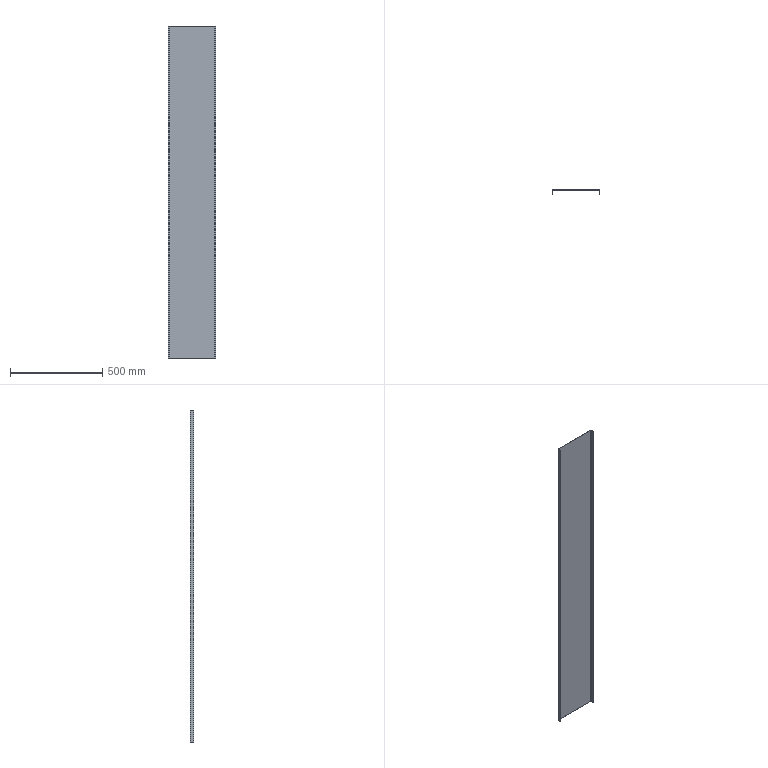Part | STEP file | 750038225 | 1 solid | 14 faces | box 255 x 21.5 x 1800 mm | volume 791285 mm3 | plane 10 | cylinder 4 | commonest cylinder face diameters 3 x2 6 x2
STEP:
#1=CARTESIAN_POINT('',(124.5,0.,900.));
#2=VERTEX_POINT('',#1);
#3=CARTESIAN_POINT('',(-124.5,0.,900.));
#4=VERTEX_POINT('',#3);
#5=CARTESIAN_POINT('',(126.,0.,900.));
#6=DIRECTION('',(-1.,0.,0.));
#7=VECTOR('',#6,1000.);
#8=LINE('',#5,#7);
#9=EDGE_CURVE('',#2,#4,#8,.T.);
#10=ORIENTED_EDGE('',*,*,#9,.T.);
#11=CARTESIAN_POINT('',(-124.5,0.,-900.));
#12=VERTEX_POINT('',#11);
#13=CARTESIAN_POINT('',(-124.5,0.,900.));
#14=DIRECTION('',(0.,0.,-1.));
#15=VECTOR('',#14,1000.);
#16=LINE('',#13,#15);
#17=EDGE_CURVE('',#4,#12,#16,.T.);
#18=ORIENTED_EDGE('',*,*,#17,.T.);
#19=CARTESIAN_POINT('',(124.5,0.,-900.));
#20=VERTEX_POINT('',#19);
#21=CARTESIAN_POINT('',(126.,0.,-900.));
#22=DIRECTION('',(1.,0.,0.));
#23=VECTOR('',#22,1000.);
#24=LINE('',#21,#23);
#25=EDGE_CURVE('',#12,#20,#24,.T.);
#26=ORIENTED_EDGE('',*,*,#25,.T.);
#27=CARTESIAN_POINT('',(124.5,0.,900.));
#28=DIRECTION('',(0.,0.,1.));
#29=VECTOR('',#28,1000.);
#30=LINE('',#27,#29);
#31=EDGE_CURVE('',#20,#2,#30,.T.);
#32=ORIENTED_EDGE('',*,*,#31,.T.);
#33=EDGE_LOOP('',(#10,#18,#26,#32));
#34=FACE_OUTER_BOUND('',#33,.T.);
#35=CARTESIAN_POINT('',(126.,0.,900.));
#36=DIRECTION('',(0.,-1.,0.));
#37=DIRECTION('',(1.,0.,0.));
#38=AXIS2_PLACEMENT_3D('',#35,#36,#37);
#39=PLANE('',#38);
#40=ADVANCED_FACE('',(#34),#39,.T.);
#41=ORIENTED_EDGE('',*,*,#17,.F.);
#42=CARTESIAN_POINT('',(-126.,-1.5,900.));
#43=VERTEX_POINT('',#42);
#44=CARTESIAN_POINT('',(-124.5,-1.5,900.));
#45=DIRECTION('',(0.,0.,-1.));
#46=DIRECTION('',(-1.,0.,0.));
#47=AXIS2_PLACEMENT_3D('',#44,#45,#46);
#48=CIRCLE('',#47,1.5);
#49=EDGE_CURVE('',#43,#4,#48,.T.);
#50=ORIENTED_EDGE('',*,*,#49,.F.);
#51=CARTESIAN_POINT('',(-126.,-1.5,-900.));
#52=VERTEX_POINT('',#51);
#53=CARTESIAN_POINT('',(-126.,-1.5,900.));
#54=DIRECTION('',(0.,0.,1.));
#55=VECTOR('',#54,1000.);
#56=LINE('',#53,#55);
#57=EDGE_CURVE('',#52,#43,#56,.T.);
#58=ORIENTED_EDGE('',*,*,#57,.F.);
#59=CARTESIAN_POINT('',(-124.5,-1.5,-900.));
#60=DIRECTION('',(0.,0.,1.));
#61=DIRECTION('',(-1.,0.,0.));
#62=AXIS2_PLACEMENT_3D('',#59,#60,#61);
#63=CIRCLE('',#62,1.5);
#64=EDGE_CURVE('',#12,#52,#63,.T.);
#65=ORIENTED_EDGE('',*,*,#64,.F.);
#66=EDGE_LOOP('',(#41,#50,#58,#65));
#67=FACE_OUTER_BOUND('',#66,.T.);
#68=CARTESIAN_POINT('',(-124.5,-1.5,900.));
#69=DIRECTION('',(0.,0.,-1.));
#70=DIRECTION('',(-1.,0.,0.));
#71=AXIS2_PLACEMENT_3D('',#68,#69,#70);
#72=CYLINDRICAL_SURFACE('',#71,1.5);
#73=ADVANCED_FACE('',(#67),#72,.F.);
#74=CARTESIAN_POINT('',(-127.5,-1.5,900.));
#75=VERTEX_POINT('',#74);
#76=CARTESIAN_POINT('',(-127.5,-20.,900.));
#77=VERTEX_POINT('',#76);
#78=CARTESIAN_POINT('',(-127.5,0.,900.));
#79=DIRECTION('',(0.,-1.,0.));
#80=VECTOR('',#79,1000.);
#81=LINE('',#78,#80);
#82=EDGE_CURVE('',#75,#77,#81,.T.);
#83=ORIENTED_EDGE('',*,*,#82,.T.);
#84=CARTESIAN_POINT('',(-126.,-20.,900.));
#85=VERTEX_POINT('',#84);
#86=CARTESIAN_POINT('',(-126.,-20.,900.));
#87=DIRECTION('',(-1.,0.,0.));
#88=VECTOR('',#87,1000.);
#89=LINE('',#86,#88);
#90=EDGE_CURVE('',#85,#77,#89,.T.);
#91=ORIENTED_EDGE('',*,*,#90,.F.);
#92=CARTESIAN_POINT('',(-126.,0.,900.));
#93=DIRECTION('',(0.,1.,0.));
#94=VECTOR('',#93,1000.);
#95=LINE('',#92,#94);
#96=EDGE_CURVE('',#85,#43,#95,.T.);
#97=ORIENTED_EDGE('',*,*,#96,.T.);
#98=ORIENTED_EDGE('',*,*,#49,.T.);
#99=ORIENTED_EDGE('',*,*,#9,.F.);
#100=CARTESIAN_POINT('',(126.,-1.5,900.));
#101=VERTEX_POINT('',#100);
#102=CARTESIAN_POINT('',(124.5,-1.5,900.));
#103=DIRECTION('',(0.,0.,-1.));
#104=DIRECTION('',(-1.,0.,0.));
#105=AXIS2_PLACEMENT_3D('',#102,#103,#104);
#106=CIRCLE('',#105,1.5);
#107=EDGE_CURVE('',#2,#101,#106,.T.);
#108=ORIENTED_EDGE('',*,*,#107,.T.);
#109=CARTESIAN_POINT('',(126.,-20.,900.));
#110=VERTEX_POINT('',#109);
#111=CARTESIAN_POINT('',(126.,0.,900.));
#112=DIRECTION('',(0.,-1.,0.));
#113=VECTOR('',#112,1000.);
#114=LINE('',#111,#113);
#115=EDGE_CURVE('',#101,#110,#114,.T.);
#116=ORIENTED_EDGE('',*,*,#115,.T.);
#117=CARTESIAN_POINT('',(127.5,-20.,900.));
#118=VERTEX_POINT('',#117);
#119=CARTESIAN_POINT('',(126.,-20.,900.));
#120=DIRECTION('',(1.,0.,0.));
#121=VECTOR('',#120,1000.);
#122=LINE('',#119,#121);
#123=EDGE_CURVE('',#110,#118,#122,.T.);
#124=ORIENTED_EDGE('',*,*,#123,.T.);
#125=CARTESIAN_POINT('',(127.5,-1.5,900.));
#126=VERTEX_POINT('',#125);
#127=CARTESIAN_POINT('',(127.5,0.,900.));
#128=DIRECTION('',(0.,1.,0.));
#129=VECTOR('',#128,1000.);
#130=LINE('',#127,#129);
#131=EDGE_CURVE('',#118,#126,#130,.T.);
#132=ORIENTED_EDGE('',*,*,#131,.T.);
#133=CARTESIAN_POINT('',(124.5,1.5,900.));
#134=VERTEX_POINT('',#133);
#135=CARTESIAN_POINT('',(124.5,-1.5,900.));
#136=DIRECTION('',(0.,0.,1.));
#137=DIRECTION('',(-1.,0.,0.));
#138=AXIS2_PLACEMENT_3D('',#135,#136,#137);
#139=CIRCLE('',#138,3.);
#140=EDGE_CURVE('',#126,#134,#139,.T.);
#141=ORIENTED_EDGE('',*,*,#140,.T.);
#142=CARTESIAN_POINT('',(-124.5,1.5,900.));
#143=VERTEX_POINT('',#142);
#144=CARTESIAN_POINT('',(-126.,1.5,900.));
#145=DIRECTION('',(-1.,0.,0.));
#146=VECTOR('',#145,1000.);
#147=LINE('',#144,#146);
#148=EDGE_CURVE('',#134,#143,#147,.T.);
#149=ORIENTED_EDGE('',*,*,#148,.T.);
#150=CARTESIAN_POINT('',(-124.5,-1.5,900.));
#151=DIRECTION('',(0.,0.,1.));
#152=DIRECTION('',(-1.,0.,0.));
#153=AXIS2_PLACEMENT_3D('',#150,#151,#152);
#154=CIRCLE('',#153,3.);
#155=EDGE_CURVE('',#143,#75,#154,.T.);
#156=ORIENTED_EDGE('',*,*,#155,.T.);
#157=EDGE_LOOP('',(#83,#91,#97,#98,#99,#108,#116,#124,#132,#141,#149,#156));
#158=FACE_OUTER_BOUND('',#157,.T.);
#159=CARTESIAN_POINT('',(-126.,0.,900.));
#160=DIRECTION('',(0.,0.,1.));
#161=DIRECTION('',(1.,0.,0.));
#162=AXIS2_PLACEMENT_3D('',#159,#160,#161);
#163=PLANE('',#162);
#164=ADVANCED_FACE('',(#158),#163,.T.);
#165=CARTESIAN_POINT('',(126.,-1.5,-900.));
#166=VERTEX_POINT('',#165);
#167=CARTESIAN_POINT('',(126.,-1.5,900.));
#168=DIRECTION('',(0.,0.,-1.));
#169=VECTOR('',#168,1000.);
#170=LINE('',#167,#169);
#171=EDGE_CURVE('',#101,#166,#170,.T.);
#172=ORIENTED_EDGE('',*,*,#171,.F.);
#173=ORIENTED_EDGE('',*,*,#107,.F.);
#174=ORIENTED_EDGE('',*,*,#31,.F.);
#175=CARTESIAN_POINT('',(124.5,-1.5,-900.));
#176=DIRECTION('',(0.,0.,1.));
#177=DIRECTION('',(-1.,0.,0.));
#178=AXIS2_PLACEMENT_3D('',#175,#176,#177);
#179=CIRCLE('',#178,1.5);
#180=EDGE_CURVE('',#166,#20,#179,.T.);
#181=ORIENTED_EDGE('',*,*,#180,.F.);
#182=EDGE_LOOP('',(#172,#173,#174,#181));
#183=FACE_OUTER_BOUND('',#182,.T.);
#184=CARTESIAN_POINT('',(124.5,-1.5,900.));
#185=DIRECTION('',(0.,0.,-1.));
#186=DIRECTION('',(-1.,0.,0.));
#187=AXIS2_PLACEMENT_3D('',#184,#185,#186);
#188=CYLINDRICAL_SURFACE('',#187,1.5);
#189=ADVANCED_FACE('',(#183),#188,.F.);
#190=ORIENTED_EDGE('',*,*,#180,.T.);
#191=ORIENTED_EDGE('',*,*,#25,.F.);
#192=ORIENTED_EDGE('',*,*,#64,.T.);
#193=CARTESIAN_POINT('',(-126.,-20.,-900.));
#194=VERTEX_POINT('',#193);
#195=CARTESIAN_POINT('',(-126.,-20.,-900.));
#196=DIRECTION('',(0.,1.,0.));
#197=VECTOR('',#196,1000.);
#198=LINE('',#195,#197);
#199=EDGE_CURVE('',#194,#52,#198,.T.);
#200=ORIENTED_EDGE('',*,*,#199,.F.);
#201=CARTESIAN_POINT('',(-127.5,-20.,-900.));
#202=VERTEX_POINT('',#201);
#203=CARTESIAN_POINT('',(-126.,-20.,-900.));
#204=DIRECTION('',(1.,0.,0.));
#205=VECTOR('',#204,1000.);
#206=LINE('',#203,#205);
#207=EDGE_CURVE('',#202,#194,#206,.T.);
#208=ORIENTED_EDGE('',*,*,#207,.F.);
#209=CARTESIAN_POINT('',(-127.5,-1.5,-900.));
#210=VERTEX_POINT('',#209);
#211=CARTESIAN_POINT('',(-127.5,-20.,-900.));
#212=DIRECTION('',(0.,-1.,0.));
#213=VECTOR('',#212,1000.);
#214=LINE('',#211,#213);
#215=EDGE_CURVE('',#210,#202,#214,.T.);
#216=ORIENTED_EDGE('',*,*,#215,.F.);
#217=CARTESIAN_POINT('',(-124.5,1.5,-900.));
#218=VERTEX_POINT('',#217);
#219=CARTESIAN_POINT('',(-124.5,-1.5,-900.));
#220=DIRECTION('',(0.,0.,1.));
#221=DIRECTION('',(-1.,0.,0.));
#222=AXIS2_PLACEMENT_3D('',#219,#220,#221);
#223=CIRCLE('',#222,3.);
#224=EDGE_CURVE('',#218,#210,#223,.T.);
#225=ORIENTED_EDGE('',*,*,#224,.F.);
#226=CARTESIAN_POINT('',(124.5,1.5,-900.));
#227=VERTEX_POINT('',#226);
#228=CARTESIAN_POINT('',(126.,1.5,-900.));
#229=DIRECTION('',(-1.,0.,0.));
#230=VECTOR('',#229,1000.);
#231=LINE('',#228,#230);
#232=EDGE_CURVE('',#227,#218,#231,.T.);
#233=ORIENTED_EDGE('',*,*,#232,.F.);
#234=CARTESIAN_POINT('',(127.5,-1.5,-900.));
#235=VERTEX_POINT('',#234);
#236=CARTESIAN_POINT('',(124.5,-1.5,-900.));
#237=DIRECTION('',(0.,0.,1.));
#238=DIRECTION('',(-1.,0.,0.));
#239=AXIS2_PLACEMENT_3D('',#236,#237,#238);
#240=CIRCLE('',#239,3.);
#241=EDGE_CURVE('',#235,#227,#240,.T.);
#242=ORIENTED_EDGE('',*,*,#241,.F.);
#243=CARTESIAN_POINT('',(127.5,-20.,-900.));
#244=VERTEX_POINT('',#243);
#245=CARTESIAN_POINT('',(127.5,-20.,-900.));
#246=DIRECTION('',(0.,1.,0.));
#247=VECTOR('',#246,1000.);
#248=LINE('',#245,#247);
#249=EDGE_CURVE('',#244,#235,#248,.T.);
#250=ORIENTED_EDGE('',*,*,#249,.F.);
#251=CARTESIAN_POINT('',(126.,-20.,-900.));
#252=VERTEX_POINT('',#251);
#253=CARTESIAN_POINT('',(126.,-20.,-900.));
#254=DIRECTION('',(-1.,0.,0.));
#255=VECTOR('',#254,1000.);
#256=LINE('',#253,#255);
#257=EDGE_CURVE('',#244,#252,#256,.T.);
#258=ORIENTED_EDGE('',*,*,#257,.T.);
#259=CARTESIAN_POINT('',(126.,-20.,-900.));
#260=DIRECTION('',(0.,-1.,0.));
#261=VECTOR('',#260,1000.);
#262=LINE('',#259,#261);
#263=EDGE_CURVE('',#166,#252,#262,.T.);
#264=ORIENTED_EDGE('',*,*,#263,.F.);
#265=EDGE_LOOP('',(#190,#191,#192,#200,#208,#216,#225,#233,#242,#250,#258,#264));
#266=FACE_OUTER_BOUND('',#265,.T.);
#267=CARTESIAN_POINT('',(126.,-20.,-900.));
#268=DIRECTION('',(0.,0.,1.));
#269=DIRECTION('',(1.,0.,0.));
#270=AXIS2_PLACEMENT_3D('',#267,#268,#269);
#271=PLANE('',#270);
#272=ADVANCED_FACE('',(#266),#271,.F.);
#273=ORIENTED_EDGE('',*,*,#96,.F.);
#274=CARTESIAN_POINT('',(-126.,-20.,900.));
#275=DIRECTION('',(0.,0.,-1.));
#276=VECTOR('',#275,1000.);
#277=LINE('',#274,#276);
#278=EDGE_CURVE('',#85,#194,#277,.T.);
#279=ORIENTED_EDGE('',*,*,#278,.T.);
#280=ORIENTED_EDGE('',*,*,#199,.T.);
#281=ORIENTED_EDGE('',*,*,#57,.T.);
#282=EDGE_LOOP('',(#273,#279,#280,#281));
#283=FACE_OUTER_BOUND('',#282,.T.);
#284=CARTESIAN_POINT('',(-126.,0.,900.));
#285=DIRECTION('',(1.,0.,0.));
#286=DIRECTION('',(0.,0.,-1.));
#287=AXIS2_PLACEMENT_3D('',#284,#285,#286);
#288=PLANE('',#287);
#289=ADVANCED_FACE('',(#283),#288,.T.);
#290=CARTESIAN_POINT('',(-127.5,-20.,900.));
#291=DIRECTION('',(0.,0.,-1.));
#292=VECTOR('',#291,1000.);
#293=LINE('',#290,#292);
#294=EDGE_CURVE('',#77,#202,#293,.T.);
#295=ORIENTED_EDGE('',*,*,#294,.F.);
#296=ORIENTED_EDGE('',*,*,#82,.F.);
#297=CARTESIAN_POINT('',(-127.5,-1.5,900.));
#298=DIRECTION('',(0.,0.,1.));
#299=VECTOR('',#298,1000.);
#300=LINE('',#297,#299);
#301=EDGE_CURVE('',#210,#75,#300,.T.);
#302=ORIENTED_EDGE('',*,*,#301,.F.);
#303=ORIENTED_EDGE('',*,*,#215,.T.);
#304=EDGE_LOOP('',(#295,#296,#302,#303));
#305=FACE_OUTER_BOUND('',#304,.T.);
#306=CARTESIAN_POINT('',(-127.5,0.,900.));
#307=DIRECTION('',(1.,0.,0.));
#308=DIRECTION('',(0.,0.,-1.));
#309=AXIS2_PLACEMENT_3D('',#306,#307,#308);
#310=PLANE('',#309);
#311=ADVANCED_FACE('',(#305),#310,.F.);
#312=ORIENTED_EDGE('',*,*,#155,.F.);
#313=CARTESIAN_POINT('',(-124.5,1.5,900.));
#314=DIRECTION('',(0.,0.,-1.));
#315=VECTOR('',#314,1000.);
#316=LINE('',#313,#315);
#317=EDGE_CURVE('',#143,#218,#316,.T.);
#318=ORIENTED_EDGE('',*,*,#317,.T.);
#319=ORIENTED_EDGE('',*,*,#224,.T.);
#320=ORIENTED_EDGE('',*,*,#301,.T.);
#321=EDGE_LOOP('',(#312,#318,#319,#320));
#322=FACE_OUTER_BOUND('',#321,.T.);
#323=CARTESIAN_POINT('',(-124.5,-1.5,900.));
#324=DIRECTION('',(0.,0.,-1.));
#325=DIRECTION('',(-1.,0.,0.));
#326=AXIS2_PLACEMENT_3D('',#323,#324,#325);
#327=CYLINDRICAL_SURFACE('',#326,3.);
#328=ADVANCED_FACE('',(#322),#327,.T.);
#329=ORIENTED_EDGE('',*,*,#317,.F.);
#330=ORIENTED_EDGE('',*,*,#148,.F.);
#331=CARTESIAN_POINT('',(124.5,1.5,900.));
#332=DIRECTION('',(0.,0.,1.));
#333=VECTOR('',#332,1000.);
#334=LINE('',#331,#333);
#335=EDGE_CURVE('',#227,#134,#334,.T.);
#336=ORIENTED_EDGE('',*,*,#335,.F.);
#337=ORIENTED_EDGE('',*,*,#232,.T.);
#338=EDGE_LOOP('',(#329,#330,#336,#337));
#339=FACE_OUTER_BOUND('',#338,.T.);
#340=CARTESIAN_POINT('',(126.,1.5,900.));
#341=DIRECTION('',(0.,-1.,0.));
#342=DIRECTION('',(1.,0.,0.));
#343=AXIS2_PLACEMENT_3D('',#340,#341,#342);
#344=PLANE('',#343);
#345=ADVANCED_FACE('',(#339),#344,.F.);
#346=ORIENTED_EDGE('',*,*,#140,.F.);
#347=CARTESIAN_POINT('',(127.5,-1.5,900.));
#348=DIRECTION('',(0.,0.,-1.));
#349=VECTOR('',#348,1000.);
#350=LINE('',#347,#349);
#351=EDGE_CURVE('',#126,#235,#350,.T.);
#352=ORIENTED_EDGE('',*,*,#351,.T.);
#353=ORIENTED_EDGE('',*,*,#241,.T.);
#354=ORIENTED_EDGE('',*,*,#335,.T.);
#355=EDGE_LOOP('',(#346,#352,#353,#354));
#356=FACE_OUTER_BOUND('',#355,.T.);
#357=CARTESIAN_POINT('',(124.5,-1.5,900.));
#358=DIRECTION('',(0.,0.,-1.));
#359=DIRECTION('',(-1.,0.,0.));
#360=AXIS2_PLACEMENT_3D('',#357,#358,#359);
#361=CYLINDRICAL_SURFACE('',#360,3.);
#362=ADVANCED_FACE('',(#356),#361,.T.);
#363=ORIENTED_EDGE('',*,*,#351,.F.);
#364=ORIENTED_EDGE('',*,*,#131,.F.);
#365=CARTESIAN_POINT('',(127.5,-20.,900.));
#366=DIRECTION('',(0.,0.,1.));
#367=VECTOR('',#366,1000.);
#368=LINE('',#365,#367);
#369=EDGE_CURVE('',#244,#118,#368,.T.);
#370=ORIENTED_EDGE('',*,*,#369,.F.);
#371=ORIENTED_EDGE('',*,*,#249,.T.);
#372=EDGE_LOOP('',(#363,#364,#370,#371));
#373=FACE_OUTER_BOUND('',#372,.T.);
#374=CARTESIAN_POINT('',(127.5,-20.,900.));
#375=DIRECTION('',(-1.,0.,0.));
#376=DIRECTION('',(0.,0.,1.));
#377=AXIS2_PLACEMENT_3D('',#374,#375,#376);
#378=PLANE('',#377);
#379=ADVANCED_FACE('',(#373),#378,.F.);
#380=ORIENTED_EDGE('',*,*,#115,.F.);
#381=ORIENTED_EDGE('',*,*,#171,.T.);
#382=ORIENTED_EDGE('',*,*,#263,.T.);
#383=CARTESIAN_POINT('',(126.,-20.,900.));
#384=DIRECTION('',(0.,0.,1.));
#385=VECTOR('',#384,1000.);
#386=LINE('',#383,#385);
#387=EDGE_CURVE('',#252,#110,#386,.T.);
#388=ORIENTED_EDGE('',*,*,#387,.T.);
#389=EDGE_LOOP('',(#380,#381,#382,#388));
#390=FACE_OUTER_BOUND('',#389,.T.);
#391=CARTESIAN_POINT('',(126.,-20.,900.));
#392=DIRECTION('',(-1.,0.,0.));
#393=DIRECTION('',(0.,0.,1.));
#394=AXIS2_PLACEMENT_3D('',#391,#392,#393);
#395=PLANE('',#394);
#396=ADVANCED_FACE('',(#390),#395,.T.);
#397=ORIENTED_EDGE('',*,*,#207,.T.);
#398=ORIENTED_EDGE('',*,*,#278,.F.);
#399=ORIENTED_EDGE('',*,*,#90,.T.);
#400=ORIENTED_EDGE('',*,*,#294,.T.);
#401=EDGE_LOOP('',(#397,#398,#399,#400));
#402=FACE_OUTER_BOUND('',#401,.T.);
#403=CARTESIAN_POINT('',(-126.,-20.,900.));
#404=DIRECTION('',(0.,-1.,0.));
#405=DIRECTION('',(0.,0.,-1.));
#406=AXIS2_PLACEMENT_3D('',#403,#404,#405);
#407=PLANE('',#406);
#408=ADVANCED_FACE('',(#402),#407,.T.);
#409=ORIENTED_EDGE('',*,*,#123,.F.);
#410=ORIENTED_EDGE('',*,*,#387,.F.);
#411=ORIENTED_EDGE('',*,*,#257,.F.);
#412=ORIENTED_EDGE('',*,*,#369,.T.);
#413=EDGE_LOOP('',(#409,#410,#411,#412));
#414=FACE_OUTER_BOUND('',#413,.T.);
#415=CARTESIAN_POINT('',(126.,-20.,900.));
#416=DIRECTION('',(0.,1.,0.));
#417=DIRECTION('',(0.,0.,1.));
#418=AXIS2_PLACEMENT_3D('',#415,#416,#417);
#419=PLANE('',#418);
#420=ADVANCED_FACE('',(#414),#419,.F.);
#421=CLOSED_SHELL('',(#40,#73,#164,#189,#272,#289,#311,#328,#345,#362,#379,#396,#408,#420));
#422=MANIFOLD_SOLID_BREP('',#421);
#423=CARTESIAN_POINT('',(0.,0.,0.));
#424=DIRECTION('',(0.,0.,1.));
#425=DIRECTION('',(1.,0.,0.));
#426=AXIS2_PLACEMENT_3D('',#423,#424,#425);
#427=(LENGTH_UNIT()NAMED_UNIT(*)SI_UNIT(.MILLI.,.METRE.));
#428=UNCERTAINTY_MEASURE_WITH_UNIT(LENGTH_MEASURE(0.00001),#427,'','');
#429=(NAMED_UNIT(*)PLANE_ANGLE_UNIT()SI_UNIT($,.RADIAN.));
#430=(NAMED_UNIT(*)SI_UNIT($,.STERADIAN.)SOLID_ANGLE_UNIT());
#431=(GEOMETRIC_REPRESENTATION_CONTEXT(3)GLOBAL_UNCERTAINTY_ASSIGNED_CONTEXT((#428))GLOBAL_UNIT_ASSIGNED_CONTEXT((#427,#429,#430))REPRESENTATION_CONTEXT('',''));
#432=ADVANCED_BREP_SHAPE_REPRESENTATION('',(#422,#426),#431);